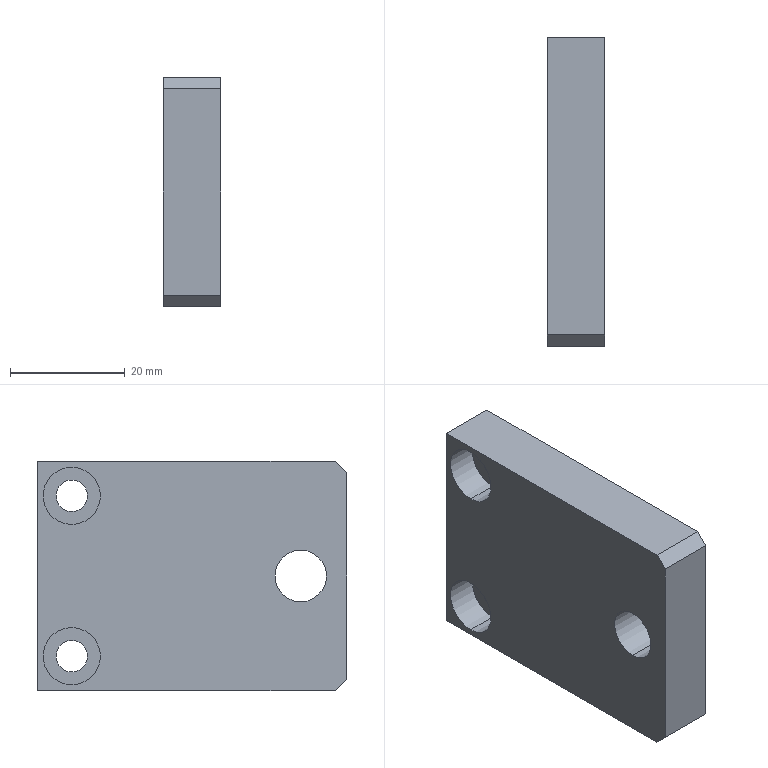Part | STEP file | PN_0007 | 1 solid | 20 faces | box 10 x 54 x 40 mm | volume 19857 mm3 | cylinder 10 | plane 10 | commonest cylinder face diameters 5.5 x4 10 x4 9 x2